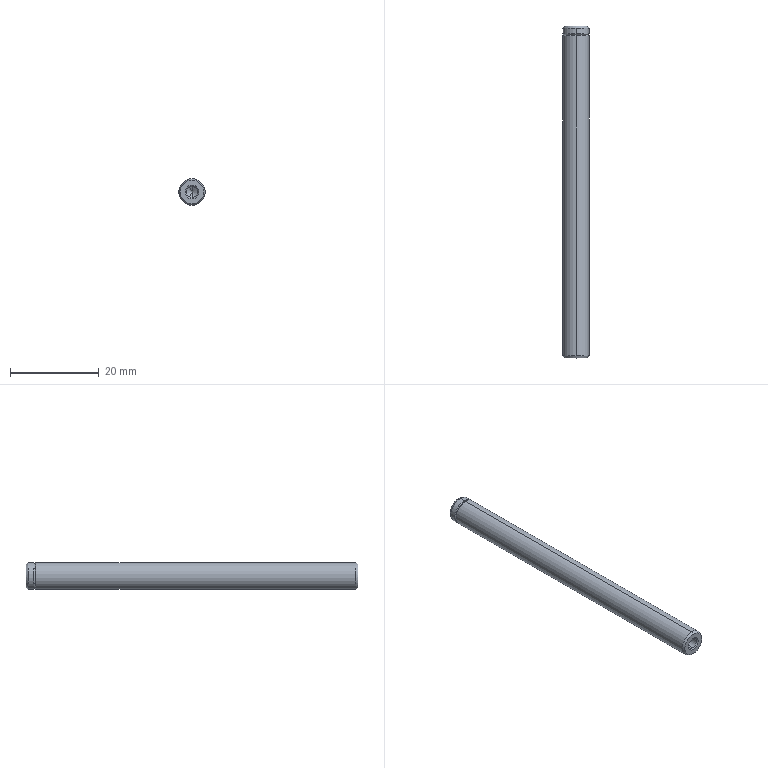Part | STEP file | MOP-75-1.step-36.STEP.STEP.STEP.STEP-548.STEP | 1 solid | 26 faces | box 6 x 75 x 6 mm | volume 2070 mm3 | cone 16 | cylinder 8 | plane 2 | commonest cylinder face diameters 2.5 x4 6 x4
STEP:
#1=CARTESIAN_POINT('',(0.,72.8,3.));
#2=VERTEX_POINT('',#1);
#3=CARTESIAN_POINT('',(0.,72.8,-3.));
#4=VERTEX_POINT('',#3);
#5=CARTESIAN_POINT('',(0.,72.8,0.));
#6=DIRECTION('',(0.,1.,0.));
#7=DIRECTION('',(0.,0.,-1.));
#8=AXIS2_PLACEMENT_3D('',#5,#6,#7);
#9=CIRCLE('',#8,3.);
#10=EDGE_CURVE('',#2,#4,#9,.T.);
#11=ORIENTED_EDGE('',*,*,#10,.F.);
#12=CARTESIAN_POINT('',(0.,0.5196,3.));
#13=VERTEX_POINT('',#12);
#14=CARTESIAN_POINT('',(0.,75.,3.));
#15=DIRECTION('',(0.,-1.,0.));
#16=VECTOR('',#15,1000.);
#17=LINE('',#14,#16);
#18=EDGE_CURVE('',#2,#13,#17,.T.);
#19=ORIENTED_EDGE('',*,*,#18,.T.);
#20=CARTESIAN_POINT('',(0.,0.5196,-3.));
#21=VERTEX_POINT('',#20);
#22=CARTESIAN_POINT('',(0.,0.5196,0.));
#23=DIRECTION('',(0.,1.,0.));
#24=DIRECTION('',(0.,0.,1.));
#25=AXIS2_PLACEMENT_3D('',#22,#23,#24);
#26=CIRCLE('',#25,3.);
#27=EDGE_CURVE('',#13,#21,#26,.T.);
#28=ORIENTED_EDGE('',*,*,#27,.T.);
#29=CARTESIAN_POINT('',(0.,75.,-3.));
#30=DIRECTION('',(0.,-1.,0.));
#31=VECTOR('',#30,1000.);
#32=LINE('',#29,#31);
#33=EDGE_CURVE('',#4,#21,#32,.T.);
#34=ORIENTED_EDGE('',*,*,#33,.F.);
#35=EDGE_LOOP('',(#11,#19,#28,#34));
#36=FACE_OUTER_BOUND('',#35,.T.);
#37=CARTESIAN_POINT('',(0.,75.,0.));
#38=DIRECTION('',(0.,-1.,0.));
#39=DIRECTION('',(0.,0.,-1.));
#40=AXIS2_PLACEMENT_3D('',#37,#38,#39);
#41=CYLINDRICAL_SURFACE('',#40,3.);
#42=ADVANCED_FACE('',(#36),#41,.T.);
#43=CARTESIAN_POINT('',(0.,0.,-2.7));
#44=VERTEX_POINT('',#43);
#45=CARTESIAN_POINT('',(0.,0.,2.7));
#46=VERTEX_POINT('',#45);
#47=CARTESIAN_POINT('',(0.,0.,0.));
#48=DIRECTION('',(0.,-1.,0.));
#49=DIRECTION('',(0.,0.,1.));
#50=AXIS2_PLACEMENT_3D('',#47,#48,#49);
#51=CIRCLE('',#50,2.7);
#52=EDGE_CURVE('',#44,#46,#51,.T.);
#53=ORIENTED_EDGE('',*,*,#52,.F.);
#54=CARTESIAN_POINT('',(0.,0.5196,-3.));
#55=DIRECTION('',(0.,0.866,-0.5));
#56=VECTOR('',#55,1000.);
#57=LINE('',#54,#56);
#58=EDGE_CURVE('',#44,#21,#57,.T.);
#59=ORIENTED_EDGE('',*,*,#58,.T.);
#60=ORIENTED_EDGE('',*,*,#27,.F.);
#61=CARTESIAN_POINT('',(0.,0.5196,3.));
#62=DIRECTION('',(0.,0.866,0.5));
#63=VECTOR('',#62,1000.);
#64=LINE('',#61,#63);
#65=EDGE_CURVE('',#46,#13,#64,.T.);
#66=ORIENTED_EDGE('',*,*,#65,.F.);
#67=EDGE_LOOP('',(#53,#59,#60,#66));
#68=FACE_OUTER_BOUND('',#67,.T.);
#69=CARTESIAN_POINT('',(0.,0.5196,0.));
#70=DIRECTION('',(0.,1.,0.));
#71=DIRECTION('',(0.,0.,1.));
#72=AXIS2_PLACEMENT_3D('',#69,#70,#71);
#73=CONICAL_SURFACE('',#72,3.,0.5236);
#74=ADVANCED_FACE('',(#68),#73,.T.);
#75=CARTESIAN_POINT('',(0.,0.3,1.25));
#76=VERTEX_POINT('',#75);
#77=CARTESIAN_POINT('',(0.,0.3,-1.25));
#78=VERTEX_POINT('',#77);
#79=CARTESIAN_POINT('',(0.,0.3,0.));
#80=DIRECTION('',(0.,-1.,0.));
#81=DIRECTION('',(0.,0.,1.));
#82=AXIS2_PLACEMENT_3D('',#79,#80,#81);
#83=CIRCLE('',#82,1.25);
#84=EDGE_CURVE('',#76,#78,#83,.T.);
#85=ORIENTED_EDGE('',*,*,#84,.F.);
#86=CARTESIAN_POINT('',(0.,0.,1.55));
#87=VERTEX_POINT('',#86);
#88=CARTESIAN_POINT('',(0.,0.3,1.25));
#89=DIRECTION('',(0.,-0.7071,0.7071));
#90=VECTOR('',#89,1000.);
#91=LINE('',#88,#90);
#92=EDGE_CURVE('',#76,#87,#91,.T.);
#93=ORIENTED_EDGE('',*,*,#92,.T.);
#94=CARTESIAN_POINT('',(0.,0.,-1.55));
#95=VERTEX_POINT('',#94);
#96=CARTESIAN_POINT('',(0.,0.,0.));
#97=DIRECTION('',(0.,1.,0.));
#98=DIRECTION('',(0.,0.,1.));
#99=AXIS2_PLACEMENT_3D('',#96,#97,#98);
#100=CIRCLE('',#99,1.55);
#101=EDGE_CURVE('',#95,#87,#100,.T.);
#102=ORIENTED_EDGE('',*,*,#101,.F.);
#103=CARTESIAN_POINT('',(0.,0.3,-1.25));
#104=DIRECTION('',(0.,-0.7071,-0.7071));
#105=VECTOR('',#104,1000.);
#106=LINE('',#103,#105);
#107=EDGE_CURVE('',#78,#95,#106,.T.);
#108=ORIENTED_EDGE('',*,*,#107,.F.);
#109=EDGE_LOOP('',(#85,#93,#102,#108));
#110=FACE_OUTER_BOUND('',#109,.T.);
#111=CARTESIAN_POINT('',(0.,0.3,0.));
#112=DIRECTION('',(0.,-1.,0.));
#113=DIRECTION('',(0.,0.,-1.));
#114=AXIS2_PLACEMENT_3D('',#111,#112,#113);
#115=CONICAL_SURFACE('',#114,1.25,0.7854);
#116=ADVANCED_FACE('',(#110),#115,.F.);
#117=CARTESIAN_POINT('',(0.,4.5,1.25));
#118=VERTEX_POINT('',#117);
#119=CARTESIAN_POINT('',(0.,4.5,-1.25));
#120=VERTEX_POINT('',#119);
#121=CARTESIAN_POINT('',(0.,4.5,0.));
#122=DIRECTION('',(0.,-1.,0.));
#123=DIRECTION('',(0.,0.,-1.));
#124=AXIS2_PLACEMENT_3D('',#121,#122,#123);
#125=CIRCLE('',#124,1.25);
#126=EDGE_CURVE('',#118,#120,#125,.T.);
#127=ORIENTED_EDGE('',*,*,#126,.F.);
#128=CARTESIAN_POINT('',(0.,0.,1.25));
#129=DIRECTION('',(0.,-1.,0.));
#130=VECTOR('',#129,1000.);
#131=LINE('',#128,#130);
#132=EDGE_CURVE('',#118,#76,#131,.T.);
#133=ORIENTED_EDGE('',*,*,#132,.T.);
#134=ORIENTED_EDGE('',*,*,#84,.T.);
#135=CARTESIAN_POINT('',(0.,0.,-1.25));
#136=DIRECTION('',(0.,-1.,0.));
#137=VECTOR('',#136,1000.);
#138=LINE('',#135,#137);
#139=EDGE_CURVE('',#120,#78,#138,.T.);
#140=ORIENTED_EDGE('',*,*,#139,.F.);
#141=EDGE_LOOP('',(#127,#133,#134,#140));
#142=FACE_OUTER_BOUND('',#141,.T.);
#143=CARTESIAN_POINT('',(0.,0.,0.));
#144=DIRECTION('',(0.,-1.,0.));
#145=DIRECTION('',(0.,0.,-1.));
#146=AXIS2_PLACEMENT_3D('',#143,#144,#145);
#147=CYLINDRICAL_SURFACE('',#146,1.25);
#148=ADVANCED_FACE('',(#142),#147,.F.);
#149=CARTESIAN_POINT('',(0.,5.251,0.));
#150=VERTEX_POINT('',#149);
#151=CARTESIAN_POINT('',(0.,4.5,-1.25));
#152=DIRECTION('',(0.,-0.515,-0.8572));
#153=VECTOR('',#152,1000.);
#154=LINE('',#151,#153);
#155=EDGE_CURVE('',#150,#120,#154,.T.);
#156=ORIENTED_EDGE('',*,*,#155,.F.);
#157=CARTESIAN_POINT('',(0.,4.5,1.25));
#158=DIRECTION('',(0.,-0.515,0.8572));
#159=VECTOR('',#158,1000.);
#160=LINE('',#157,#159);
#161=EDGE_CURVE('',#150,#118,#160,.T.);
#162=ORIENTED_EDGE('',*,*,#161,.T.);
#163=ORIENTED_EDGE('',*,*,#126,.T.);
#164=EDGE_LOOP('',(#156,#162,#163));
#165=FACE_OUTER_BOUND('',#164,.T.);
#166=CARTESIAN_POINT('',(0.,4.5,0.));
#167=DIRECTION('',(0.,-1.,0.));
#168=DIRECTION('',(0.,0.,-1.));
#169=AXIS2_PLACEMENT_3D('',#166,#167,#168);
#170=CONICAL_SURFACE('',#169,1.25,1.03);
#171=ADVANCED_FACE('',(#165),#170,.F.);
#172=CARTESIAN_POINT('',(0.,73.,-2.8));
#173=VERTEX_POINT('',#172);
#174=CARTESIAN_POINT('',(0.,73.,2.8));
#175=VERTEX_POINT('',#174);
#176=CARTESIAN_POINT('',(0.,73.,0.));
#177=DIRECTION('',(0.,-1.,0.));
#178=DIRECTION('',(0.,0.,-1.));
#179=AXIS2_PLACEMENT_3D('',#176,#177,#178);
#180=CIRCLE('',#179,2.8);
#181=EDGE_CURVE('',#173,#175,#180,.T.);
#182=ORIENTED_EDGE('',*,*,#181,.T.);
#183=CARTESIAN_POINT('',(0.,-110.306,186.106));
#184=DIRECTION('',(0.,-0.7071,0.7071));
#185=VECTOR('',#184,1000.);
#186=LINE('',#183,#185);
#187=EDGE_CURVE('',#175,#2,#186,.T.);
#188=ORIENTED_EDGE('',*,*,#187,.T.);
#189=ORIENTED_EDGE('',*,*,#10,.T.);
#190=CARTESIAN_POINT('',(0.,-110.306,-186.106));
#191=DIRECTION('',(0.,-0.7071,-0.7071));
#192=VECTOR('',#191,1000.);
#193=LINE('',#190,#192);
#194=EDGE_CURVE('',#173,#4,#193,.T.);
#195=ORIENTED_EDGE('',*,*,#194,.F.);
#196=EDGE_LOOP('',(#182,#188,#189,#195));
#197=FACE_OUTER_BOUND('',#196,.T.);
#198=CARTESIAN_POINT('',(0.,-110.306,0.));
#199=DIRECTION('',(0.,-1.,0.));
#200=DIRECTION('',(0.,0.,-1.));
#201=AXIS2_PLACEMENT_3D('',#198,#199,#200);
#202=CONICAL_SURFACE('',#201,186.106,0.7854);
#203=ADVANCED_FACE('',(#197),#202,.T.);
#204=ORIENTED_EDGE('',*,*,#181,.F.);
#205=CARTESIAN_POINT('',(0.,73.2,-3.));
#206=VERTEX_POINT('',#205);
#207=CARTESIAN_POINT('',(0.,73.,-2.8));
#208=DIRECTION('',(0.,0.7071,-0.7071));
#209=VECTOR('',#208,1000.);
#210=LINE('',#207,#209);
#211=EDGE_CURVE('',#173,#206,#210,.T.);
#212=ORIENTED_EDGE('',*,*,#211,.T.);
#213=CARTESIAN_POINT('',(0.,73.2,3.));
#214=VERTEX_POINT('',#213);
#215=CARTESIAN_POINT('',(0.,73.2,0.));
#216=DIRECTION('',(0.,-1.,0.));
#217=DIRECTION('',(0.,0.,1.));
#218=AXIS2_PLACEMENT_3D('',#215,#216,#217);
#219=CIRCLE('',#218,3.);
#220=EDGE_CURVE('',#206,#214,#219,.T.);
#221=ORIENTED_EDGE('',*,*,#220,.T.);
#222=CARTESIAN_POINT('',(0.,73.,2.8));
#223=DIRECTION('',(0.,0.7071,0.7071));
#224=VECTOR('',#223,1000.);
#225=LINE('',#222,#224);
#226=EDGE_CURVE('',#175,#214,#225,.T.);
#227=ORIENTED_EDGE('',*,*,#226,.F.);
#228=EDGE_LOOP('',(#204,#212,#221,#227));
#229=FACE_OUTER_BOUND('',#228,.T.);
#230=CARTESIAN_POINT('',(0.,73.,0.));
#231=DIRECTION('',(0.,1.,0.));
#232=DIRECTION('',(0.,0.,1.));
#233=AXIS2_PLACEMENT_3D('',#230,#231,#232);
#234=CONICAL_SURFACE('',#233,2.8,0.7854);
#235=ADVANCED_FACE('',(#229),#234,.T.);
#236=CARTESIAN_POINT('',(0.,74.7,-1.25));
#237=VERTEX_POINT('',#236);
#238=CARTESIAN_POINT('',(0.,74.7,1.25));
#239=VERTEX_POINT('',#238);
#240=CARTESIAN_POINT('',(0.,74.7,0.));
#241=DIRECTION('',(0.,1.,0.));
#242=DIRECTION('',(0.,0.,1.));
#243=AXIS2_PLACEMENT_3D('',#240,#241,#242);
#244=CIRCLE('',#243,1.25);
#245=EDGE_CURVE('',#237,#239,#244,.T.);
#246=ORIENTED_EDGE('',*,*,#245,.F.);
#247=CARTESIAN_POINT('',(0.,75.,-1.55));
#248=VERTEX_POINT('',#247);
#249=CARTESIAN_POINT('',(0.,74.7,-1.25));
#250=DIRECTION('',(0.,0.7071,-0.7071));
#251=VECTOR('',#250,1000.);
#252=LINE('',#249,#251);
#253=EDGE_CURVE('',#237,#248,#252,.T.);
#254=ORIENTED_EDGE('',*,*,#253,.T.);
#255=CARTESIAN_POINT('',(0.,75.,1.55));
#256=VERTEX_POINT('',#255);
#257=CARTESIAN_POINT('',(0.,75.,0.));
#258=DIRECTION('',(0.,-1.,0.));
#259=DIRECTION('',(0.,0.,1.));
#260=AXIS2_PLACEMENT_3D('',#257,#258,#259);
#261=CIRCLE('',#260,1.55);
#262=EDGE_CURVE('',#256,#248,#261,.T.);
#263=ORIENTED_EDGE('',*,*,#262,.F.);
#264=CARTESIAN_POINT('',(0.,74.7,1.25));
#265=DIRECTION('',(0.,0.7071,0.7071));
#266=VECTOR('',#265,1000.);
#267=LINE('',#264,#266);
#268=EDGE_CURVE('',#239,#256,#267,.T.);
#269=ORIENTED_EDGE('',*,*,#268,.F.);
#270=EDGE_LOOP('',(#246,#254,#263,#269));
#271=FACE_OUTER_BOUND('',#270,.T.);
#272=CARTESIAN_POINT('',(0.,74.7,0.));
#273=DIRECTION('',(0.,1.,0.));
#274=DIRECTION('',(0.,0.,1.));
#275=AXIS2_PLACEMENT_3D('',#272,#273,#274);
#276=CONICAL_SURFACE('',#275,1.25,0.7854);
#277=ADVANCED_FACE('',(#271),#276,.F.);
#278=CARTESIAN_POINT('',(0.,75.,2.7));
#279=VERTEX_POINT('',#278);
#280=CARTESIAN_POINT('',(0.,75.,-2.7));
#281=VERTEX_POINT('',#280);
#282=CARTESIAN_POINT('',(0.,75.,0.));
#283=DIRECTION('',(0.,1.,0.));
#284=DIRECTION('',(0.,0.,1.));
#285=AXIS2_PLACEMENT_3D('',#282,#283,#284);
#286=CIRCLE('',#285,2.7);
#287=EDGE_CURVE('',#279,#281,#286,.T.);
#288=ORIENTED_EDGE('',*,*,#287,.F.);
#289=CARTESIAN_POINT('',(0.,74.48,3.));
#290=VERTEX_POINT('',#289);
#291=CARTESIAN_POINT('',(0.,75.,2.7));
#292=DIRECTION('',(0.,-0.866,0.5));
#293=VECTOR('',#292,1000.);
#294=LINE('',#291,#293);
#295=EDGE_CURVE('',#279,#290,#294,.T.);
#296=ORIENTED_EDGE('',*,*,#295,.T.);
#297=CARTESIAN_POINT('',(0.,74.48,-3.));
#298=VERTEX_POINT('',#297);
#299=CARTESIAN_POINT('',(0.,74.48,0.));
#300=DIRECTION('',(0.,-1.,0.));
#301=DIRECTION('',(0.,0.,1.));
#302=AXIS2_PLACEMENT_3D('',#299,#300,#301);
#303=CIRCLE('',#302,3.);
#304=EDGE_CURVE('',#298,#290,#303,.T.);
#305=ORIENTED_EDGE('',*,*,#304,.F.);
#306=CARTESIAN_POINT('',(0.,75.,-2.7));
#307=DIRECTION('',(0.,-0.866,-0.5));
#308=VECTOR('',#307,1000.);
#309=LINE('',#306,#308);
#310=EDGE_CURVE('',#281,#298,#309,.T.);
#311=ORIENTED_EDGE('',*,*,#310,.F.);
#312=EDGE_LOOP('',(#288,#296,#305,#311));
#313=FACE_OUTER_BOUND('',#312,.T.);
#314=CARTESIAN_POINT('',(0.,75.,0.));
#315=DIRECTION('',(0.,-1.,0.));
#316=DIRECTION('',(0.,0.,-1.));
#317=AXIS2_PLACEMENT_3D('',#314,#315,#316);
#318=CONICAL_SURFACE('',#317,2.7,0.5236);
#319=ADVANCED_FACE('',(#313),#318,.T.);
#320=CARTESIAN_POINT('',(0.,70.5,-1.25));
#321=VERTEX_POINT('',#320);
#322=CARTESIAN_POINT('',(0.,70.5,1.25));
#323=VERTEX_POINT('',#322);
#324=CARTESIAN_POINT('',(0.,70.5,0.));
#325=DIRECTION('',(0.,1.,0.));
#326=DIRECTION('',(0.,0.,1.));
#327=AXIS2_PLACEMENT_3D('',#324,#325,#326);
#328=CIRCLE('',#327,1.25);
#329=EDGE_CURVE('',#321,#323,#328,.T.);
#330=ORIENTED_EDGE('',*,*,#329,.F.);
#331=CARTESIAN_POINT('',(0.,75.,-1.25));
#332=DIRECTION('',(0.,1.,0.));
#333=VECTOR('',#332,1000.);
#334=LINE('',#331,#333);
#335=EDGE_CURVE('',#321,#237,#334,.T.);
#336=ORIENTED_EDGE('',*,*,#335,.T.);
#337=ORIENTED_EDGE('',*,*,#245,.T.);
#338=CARTESIAN_POINT('',(0.,75.,1.25));
#339=DIRECTION('',(0.,1.,0.));
#340=VECTOR('',#339,1000.);
#341=LINE('',#338,#340);
#342=EDGE_CURVE('',#323,#239,#341,.T.);
#343=ORIENTED_EDGE('',*,*,#342,.F.);
#344=EDGE_LOOP('',(#330,#336,#337,#343));
#345=FACE_OUTER_BOUND('',#344,.T.);
#346=CARTESIAN_POINT('',(0.,75.,0.));
#347=DIRECTION('',(0.,1.,0.));
#348=DIRECTION('',(0.,0.,1.));
#349=AXIS2_PLACEMENT_3D('',#346,#347,#348);
#350=CYLINDRICAL_SURFACE('',#349,1.25);
#351=ADVANCED_FACE('',(#345),#350,.F.);
#352=CARTESIAN_POINT('',(0.,69.749,0.));
#353=VERTEX_POINT('',#352);
#354=CARTESIAN_POINT('',(0.,70.5,1.25));
#355=DIRECTION('',(0.,0.515,0.8572));
#356=VECTOR('',#355,1000.);
#357=LINE('',#354,#356);
#358=EDGE_CURVE('',#353,#323,#357,.T.);
#359=ORIENTED_EDGE('',*,*,#358,.F.);
#360=CARTESIAN_POINT('',(0.,70.5,-1.25));
#361=DIRECTION('',(0.,0.515,-0.8572));
#362=VECTOR('',#361,1000.);
#363=LINE('',#360,#362);
#364=EDGE_CURVE('',#353,#321,#363,.T.);
#365=ORIENTED_EDGE('',*,*,#364,.T.);
#366=ORIENTED_EDGE('',*,*,#329,.T.);
#367=EDGE_LOOP('',(#359,#365,#366));
#368=FACE_OUTER_BOUND('',#367,.T.);
#369=CARTESIAN_POINT('',(0.,70.5,0.));
#370=DIRECTION('',(0.,1.,0.));
#371=DIRECTION('',(0.,0.,1.));
#372=AXIS2_PLACEMENT_3D('',#369,#370,#371);
#373=CONICAL_SURFACE('',#372,1.25,1.03);
#374=ADVANCED_FACE('',(#368),#373,.F.);
#375=ORIENTED_EDGE('',*,*,#304,.T.);
#376=CARTESIAN_POINT('',(0.,75.,3.));
#377=DIRECTION('',(0.,-1.,0.));
#378=VECTOR('',#377,1000.);
#379=LINE('',#376,#378);
#380=EDGE_CURVE('',#290,#214,#379,.T.);
#381=ORIENTED_EDGE('',*,*,#380,.T.);
#382=ORIENTED_EDGE('',*,*,#220,.F.);
#383=CARTESIAN_POINT('',(0.,75.,-3.));
#384=DIRECTION('',(0.,-1.,0.));
#385=VECTOR('',#384,1000.);
#386=LINE('',#383,#385);
#387=EDGE_CURVE('',#298,#206,#386,.T.);
#388=ORIENTED_EDGE('',*,*,#387,.F.);
#389=EDGE_LOOP('',(#375,#381,#382,#388));
#390=FACE_OUTER_BOUND('',#389,.T.);
#391=CARTESIAN_POINT('',(0.,75.,0.));
#392=DIRECTION('',(0.,-1.,0.));
#393=DIRECTION('',(0.,0.,-1.));
#394=AXIS2_PLACEMENT_3D('',#391,#392,#393);
#395=CYLINDRICAL_SURFACE('',#394,3.);
#396=ADVANCED_FACE('',(#390),#395,.T.);
#397=ORIENTED_EDGE('',*,*,#380,.F.);
#398=CARTESIAN_POINT('',(0.,74.48,0.));
#399=DIRECTION('',(0.,-1.,0.));
#400=DIRECTION('',(0.,0.,1.));
#401=AXIS2_PLACEMENT_3D('',#398,#399,#400);
#402=CIRCLE('',#401,3.);
#403=EDGE_CURVE('',#290,#298,#402,.T.);
#404=ORIENTED_EDGE('',*,*,#403,.T.);
#405=ORIENTED_EDGE('',*,*,#387,.T.);
#406=CARTESIAN_POINT('',(0.,73.2,0.));
#407=DIRECTION('',(0.,-1.,0.));
#408=DIRECTION('',(0.,0.,1.));
#409=AXIS2_PLACEMENT_3D('',#406,#407,#408);
#410=CIRCLE('',#409,3.);
#411=EDGE_CURVE('',#214,#206,#410,.T.);
#412=ORIENTED_EDGE('',*,*,#411,.F.);
#413=EDGE_LOOP('',(#397,#404,#405,#412));
#414=FACE_OUTER_BOUND('',#413,.T.);
#415=CARTESIAN_POINT('',(0.,75.,0.));
#416=DIRECTION('',(0.,-1.,0.));
#417=DIRECTION('',(0.,0.,-1.));
#418=AXIS2_PLACEMENT_3D('',#415,#416,#417);
#419=CYLINDRICAL_SURFACE('',#418,3.);
#420=ADVANCED_FACE('',(#414),#419,.T.);
#421=ORIENTED_EDGE('',*,*,#262,.T.);
#422=CARTESIAN_POINT('',(0.,75.,0.));
#423=DIRECTION('',(0.,-1.,0.));
#424=DIRECTION('',(0.,0.,1.));
#425=AXIS2_PLACEMENT_3D('',#422,#423,#424);
#426=CIRCLE('',#425,1.55);
#427=EDGE_CURVE('',#248,#256,#426,.T.);
#428=ORIENTED_EDGE('',*,*,#427,.T.);
#429=EDGE_LOOP('',(#421,#428));
#430=FACE_BOUND('',#429,.T.);
#431=CARTESIAN_POINT('',(0.,75.,0.));
#432=DIRECTION('',(0.,1.,0.));
#433=DIRECTION('',(0.,0.,1.));
#434=AXIS2_PLACEMENT_3D('',#431,#432,#433);
#435=CIRCLE('',#434,2.7);
#436=EDGE_CURVE('',#281,#279,#435,.T.);
#437=ORIENTED_EDGE('',*,*,#436,.T.);
#438=ORIENTED_EDGE('',*,*,#287,.T.);
#439=EDGE_LOOP('',(#437,#438));
#440=FACE_OUTER_BOUND('',#439,.T.);
#441=CARTESIAN_POINT('',(0.,75.,0.));
#442=DIRECTION('',(0.,1.,0.));
#443=DIRECTION('',(1.,0.,0.));
#444=AXIS2_PLACEMENT_3D('',#441,#442,#443);
#445=PLANE('',#444);
#446=ADVANCED_FACE('',(#430,#440),#445,.T.);
#447=ORIENTED_EDGE('',*,*,#364,.F.);
#448=ORIENTED_EDGE('',*,*,#358,.T.);
#449=CARTESIAN_POINT('',(0.,70.5,0.));
#450=DIRECTION('',(0.,1.,0.));
#451=DIRECTION('',(0.,0.,1.));
#452=AXIS2_PLACEMENT_3D('',#449,#450,#451);
#453=CIRCLE('',#452,1.25);
#454=EDGE_CURVE('',#323,#321,#453,.T.);
#455=ORIENTED_EDGE('',*,*,#454,.T.);
#456=EDGE_LOOP('',(#447,#448,#455));
#457=FACE_OUTER_BOUND('',#456,.T.);
#458=CARTESIAN_POINT('',(0.,70.5,0.));
#459=DIRECTION('',(0.,1.,0.));
#460=DIRECTION('',(0.,0.,1.));
#461=AXIS2_PLACEMENT_3D('',#458,#459,#460);
#462=CONICAL_SURFACE('',#461,1.25,1.03);
#463=ADVANCED_FACE('',(#457),#462,.F.);
#464=ORIENTED_EDGE('',*,*,#335,.F.);
#465=ORIENTED_EDGE('',*,*,#454,.F.);
#466=ORIENTED_EDGE('',*,*,#342,.T.);
#467=CARTESIAN_POINT('',(0.,74.7,0.));
#468=DIRECTION('',(0.,1.,0.));
#469=DIRECTION('',(0.,0.,1.));
#470=AXIS2_PLACEMENT_3D('',#467,#468,#469);
#471=CIRCLE('',#470,1.25);
#472=EDGE_CURVE('',#239,#237,#471,.T.);
#473=ORIENTED_EDGE('',*,*,#472,.T.);
#474=EDGE_LOOP('',(#464,#465,#466,#473));
#475=FACE_OUTER_BOUND('',#474,.T.);
#476=CARTESIAN_POINT('',(0.,75.,0.));
#477=DIRECTION('',(0.,1.,0.));
#478=DIRECTION('',(0.,0.,1.));
#479=AXIS2_PLACEMENT_3D('',#476,#477,#478);
#480=CYLINDRICAL_SURFACE('',#479,1.25);
#481=ADVANCED_FACE('',(#475),#480,.F.);
#482=ORIENTED_EDGE('',*,*,#295,.F.);
#483=ORIENTED_EDGE('',*,*,#436,.F.);
#484=ORIENTED_EDGE('',*,*,#310,.T.);
#485=ORIENTED_EDGE('',*,*,#403,.F.);
#486=EDGE_LOOP('',(#482,#483,#484,#485));
#487=FACE_OUTER_BOUND('',#486,.T.);
#488=CARTESIAN_POINT('',(0.,75.,0.));
#489=DIRECTION('',(0.,-1.,0.));
#490=DIRECTION('',(0.,0.,-1.));
#491=AXIS2_PLACEMENT_3D('',#488,#489,#490);
#492=CONICAL_SURFACE('',#491,2.7,0.5236);
#493=ADVANCED_FACE('',(#487),#492,.T.);
#494=ORIENTED_EDGE('',*,*,#253,.F.);
#495=ORIENTED_EDGE('',*,*,#472,.F.);
#496=ORIENTED_EDGE('',*,*,#268,.T.);
#497=ORIENTED_EDGE('',*,*,#427,.F.);
#498=EDGE_LOOP('',(#494,#495,#496,#497));
#499=FACE_OUTER_BOUND('',#498,.T.);
#500=CARTESIAN_POINT('',(0.,74.7,0.));
#501=DIRECTION('',(0.,1.,0.));
#502=DIRECTION('',(0.,0.,1.));
#503=AXIS2_PLACEMENT_3D('',#500,#501,#502);
#504=CONICAL_SURFACE('',#503,1.25,0.7854);
#505=ADVANCED_FACE('',(#499),#504,.F.);
#506=ORIENTED_EDGE('',*,*,#211,.F.);
#507=CARTESIAN_POINT('',(0.,73.,0.));
#508=DIRECTION('',(0.,-1.,0.));
#509=DIRECTION('',(0.,0.,-1.));
#510=AXIS2_PLACEMENT_3D('',#507,#508,#509);
#511=CIRCLE('',#510,2.8);
#512=EDGE_CURVE('',#175,#173,#511,.T.);
#513=ORIENTED_EDGE('',*,*,#512,.F.);
#514=ORIENTED_EDGE('',*,*,#226,.T.);
#515=ORIENTED_EDGE('',*,*,#411,.T.);
#516=EDGE_LOOP('',(#506,#513,#514,#515));
#517=FACE_OUTER_BOUND('',#516,.T.);
#518=CARTESIAN_POINT('',(0.,73.,0.));
#519=DIRECTION('',(0.,1.,0.));
#520=DIRECTION('',(0.,0.,1.));
#521=AXIS2_PLACEMENT_3D('',#518,#519,#520);
#522=CONICAL_SURFACE('',#521,2.8,0.7854);
#523=ADVANCED_FACE('',(#517),#522,.T.);
#524=ORIENTED_EDGE('',*,*,#187,.F.);
#525=ORIENTED_EDGE('',*,*,#512,.T.);
#526=ORIENTED_EDGE('',*,*,#194,.T.);
#527=CARTESIAN_POINT('',(0.,72.8,0.));
#528=DIRECTION('',(0.,1.,0.));
#529=DIRECTION('',(0.,0.,-1.));
#530=AXIS2_PLACEMENT_3D('',#527,#528,#529);
#531=CIRCLE('',#530,3.);
#532=EDGE_CURVE('',#4,#2,#531,.T.);
#533=ORIENTED_EDGE('',*,*,#532,.T.);
#534=EDGE_LOOP('',(#524,#525,#526,#533));
#535=FACE_OUTER_BOUND('',#534,.T.);
#536=CARTESIAN_POINT('',(0.,-110.306,0.));
#537=DIRECTION('',(0.,-1.,0.));
#538=DIRECTION('',(0.,0.,-1.));
#539=AXIS2_PLACEMENT_3D('',#536,#537,#538);
#540=CONICAL_SURFACE('',#539,186.106,0.7854);
#541=ADVANCED_FACE('',(#535),#540,.T.);
#542=ORIENTED_EDGE('',*,*,#161,.F.);
#543=ORIENTED_EDGE('',*,*,#155,.T.);
#544=CARTESIAN_POINT('',(0.,4.5,0.));
#545=DIRECTION('',(0.,-1.,0.));
#546=DIRECTION('',(0.,0.,-1.));
#547=AXIS2_PLACEMENT_3D('',#544,#545,#546);
#548=CIRCLE('',#547,1.25);
#549=EDGE_CURVE('',#120,#118,#548,.T.);
#550=ORIENTED_EDGE('',*,*,#549,.T.);
#551=EDGE_LOOP('',(#542,#543,#550));
#552=FACE_OUTER_BOUND('',#551,.T.);
#553=CARTESIAN_POINT('',(0.,4.5,0.));
#554=DIRECTION('',(0.,-1.,0.));
#555=DIRECTION('',(0.,0.,-1.));
#556=AXIS2_PLACEMENT_3D('',#553,#554,#555);
#557=CONICAL_SURFACE('',#556,1.25,1.03);
#558=ADVANCED_FACE('',(#552),#557,.F.);
#559=ORIENTED_EDGE('',*,*,#132,.F.);
#560=ORIENTED_EDGE('',*,*,#549,.F.);
#561=ORIENTED_EDGE('',*,*,#139,.T.);
#562=CARTESIAN_POINT('',(0.,0.3,0.));
#563=DIRECTION('',(0.,-1.,0.));
#564=DIRECTION('',(0.,0.,1.));
#565=AXIS2_PLACEMENT_3D('',#562,#563,#564);
#566=CIRCLE('',#565,1.25);
#567=EDGE_CURVE('',#78,#76,#566,.T.);
#568=ORIENTED_EDGE('',*,*,#567,.T.);
#569=EDGE_LOOP('',(#559,#560,#561,#568));
#570=FACE_OUTER_BOUND('',#569,.T.);
#571=CARTESIAN_POINT('',(0.,0.,0.));
#572=DIRECTION('',(0.,-1.,0.));
#573=DIRECTION('',(0.,0.,-1.));
#574=AXIS2_PLACEMENT_3D('',#571,#572,#573);
#575=CYLINDRICAL_SURFACE('',#574,1.25);
#576=ADVANCED_FACE('',(#570),#575,.F.);
#577=ORIENTED_EDGE('',*,*,#92,.F.);
#578=ORIENTED_EDGE('',*,*,#567,.F.);
#579=ORIENTED_EDGE('',*,*,#107,.T.);
#580=CARTESIAN_POINT('',(0.,0.,0.));
#581=DIRECTION('',(0.,1.,0.));
#582=DIRECTION('',(0.,0.,1.));
#583=AXIS2_PLACEMENT_3D('',#580,#581,#582);
#584=CIRCLE('',#583,1.55);
#585=EDGE_CURVE('',#87,#95,#584,.T.);
#586=ORIENTED_EDGE('',*,*,#585,.F.);
#587=EDGE_LOOP('',(#577,#578,#579,#586));
#588=FACE_OUTER_BOUND('',#587,.T.);
#589=CARTESIAN_POINT('',(0.,0.3,0.));
#590=DIRECTION('',(0.,-1.,0.));
#591=DIRECTION('',(0.,0.,-1.));
#592=AXIS2_PLACEMENT_3D('',#589,#590,#591);
#593=CONICAL_SURFACE('',#592,1.25,0.7854);
#594=ADVANCED_FACE('',(#588),#593,.F.);
#595=ORIENTED_EDGE('',*,*,#101,.T.);
#596=ORIENTED_EDGE('',*,*,#585,.T.);
#597=EDGE_LOOP('',(#595,#596));
#598=FACE_BOUND('',#597,.T.);
#599=CARTESIAN_POINT('',(0.,0.,0.));
#600=DIRECTION('',(0.,-1.,0.));
#601=DIRECTION('',(0.,0.,1.));
#602=AXIS2_PLACEMENT_3D('',#599,#600,#601);
#603=CIRCLE('',#602,2.7);
#604=EDGE_CURVE('',#46,#44,#603,.T.);
#605=ORIENTED_EDGE('',*,*,#604,.T.);
#606=ORIENTED_EDGE('',*,*,#52,.T.);
#607=EDGE_LOOP('',(#605,#606));
#608=FACE_OUTER_BOUND('',#607,.T.);
#609=CARTESIAN_POINT('',(0.,0.,0.));
#610=DIRECTION('',(0.,1.,0.));
#611=DIRECTION('',(1.,0.,0.));
#612=AXIS2_PLACEMENT_3D('',#609,#610,#611);
#613=PLANE('',#612);
#614=ADVANCED_FACE('',(#598,#608),#613,.F.);
#615=ORIENTED_EDGE('',*,*,#58,.F.);
#616=ORIENTED_EDGE('',*,*,#604,.F.);
#617=ORIENTED_EDGE('',*,*,#65,.T.);
#618=CARTESIAN_POINT('',(0.,0.5196,0.));
#619=DIRECTION('',(0.,1.,0.));
#620=DIRECTION('',(0.,0.,1.));
#621=AXIS2_PLACEMENT_3D('',#618,#619,#620);
#622=CIRCLE('',#621,3.);
#623=EDGE_CURVE('',#21,#13,#622,.T.);
#624=ORIENTED_EDGE('',*,*,#623,.F.);
#625=EDGE_LOOP('',(#615,#616,#617,#624));
#626=FACE_OUTER_BOUND('',#625,.T.);
#627=CARTESIAN_POINT('',(0.,0.5196,0.));
#628=DIRECTION('',(0.,1.,0.));
#629=DIRECTION('',(0.,0.,1.));
#630=AXIS2_PLACEMENT_3D('',#627,#628,#629);
#631=CONICAL_SURFACE('',#630,3.,0.5236);
#632=ADVANCED_FACE('',(#626),#631,.T.);
#633=ORIENTED_EDGE('',*,*,#18,.F.);
#634=ORIENTED_EDGE('',*,*,#532,.F.);
#635=ORIENTED_EDGE('',*,*,#33,.T.);
#636=ORIENTED_EDGE('',*,*,#623,.T.);
#637=EDGE_LOOP('',(#633,#634,#635,#636));
#638=FACE_OUTER_BOUND('',#637,.T.);
#639=CARTESIAN_POINT('',(0.,75.,0.));
#640=DIRECTION('',(0.,-1.,0.));
#641=DIRECTION('',(0.,0.,-1.));
#642=AXIS2_PLACEMENT_3D('',#639,#640,#641);
#643=CYLINDRICAL_SURFACE('',#642,3.);
#644=ADVANCED_FACE('',(#638),#643,.T.);
#645=CLOSED_SHELL('',(#42,#74,#116,#148,#171,#203,#235,#277,#319,#351,#374,#396,#420,#446,#463,#481,#493,#505,#523,#541,#558,#576,#594,#614,#632,#644));
#646=MANIFOLD_SOLID_BREP('',#645);
#647=CARTESIAN_POINT('',(0.,0.,0.));
#648=DIRECTION('',(0.,0.,1.));
#649=DIRECTION('',(1.,0.,0.));
#650=AXIS2_PLACEMENT_3D('',#647,#648,#649);
#651=(LENGTH_UNIT()NAMED_UNIT(*)SI_UNIT(.MILLI.,.METRE.));
#652=UNCERTAINTY_MEASURE_WITH_UNIT(LENGTH_MEASURE(0.00001),#651,'','');
#653=(NAMED_UNIT(*)PLANE_ANGLE_UNIT()SI_UNIT($,.RADIAN.));
#654=(NAMED_UNIT(*)SI_UNIT($,.STERADIAN.)SOLID_ANGLE_UNIT());
#655=(GEOMETRIC_REPRESENTATION_CONTEXT(3)GLOBAL_UNCERTAINTY_ASSIGNED_CONTEXT((#652))GLOBAL_UNIT_ASSIGNED_CONTEXT((#651,#653,#654))REPRESENTATION_CONTEXT('',''));
#656=ADVANCED_BREP_SHAPE_REPRESENTATION('',(#646,#650),#655);